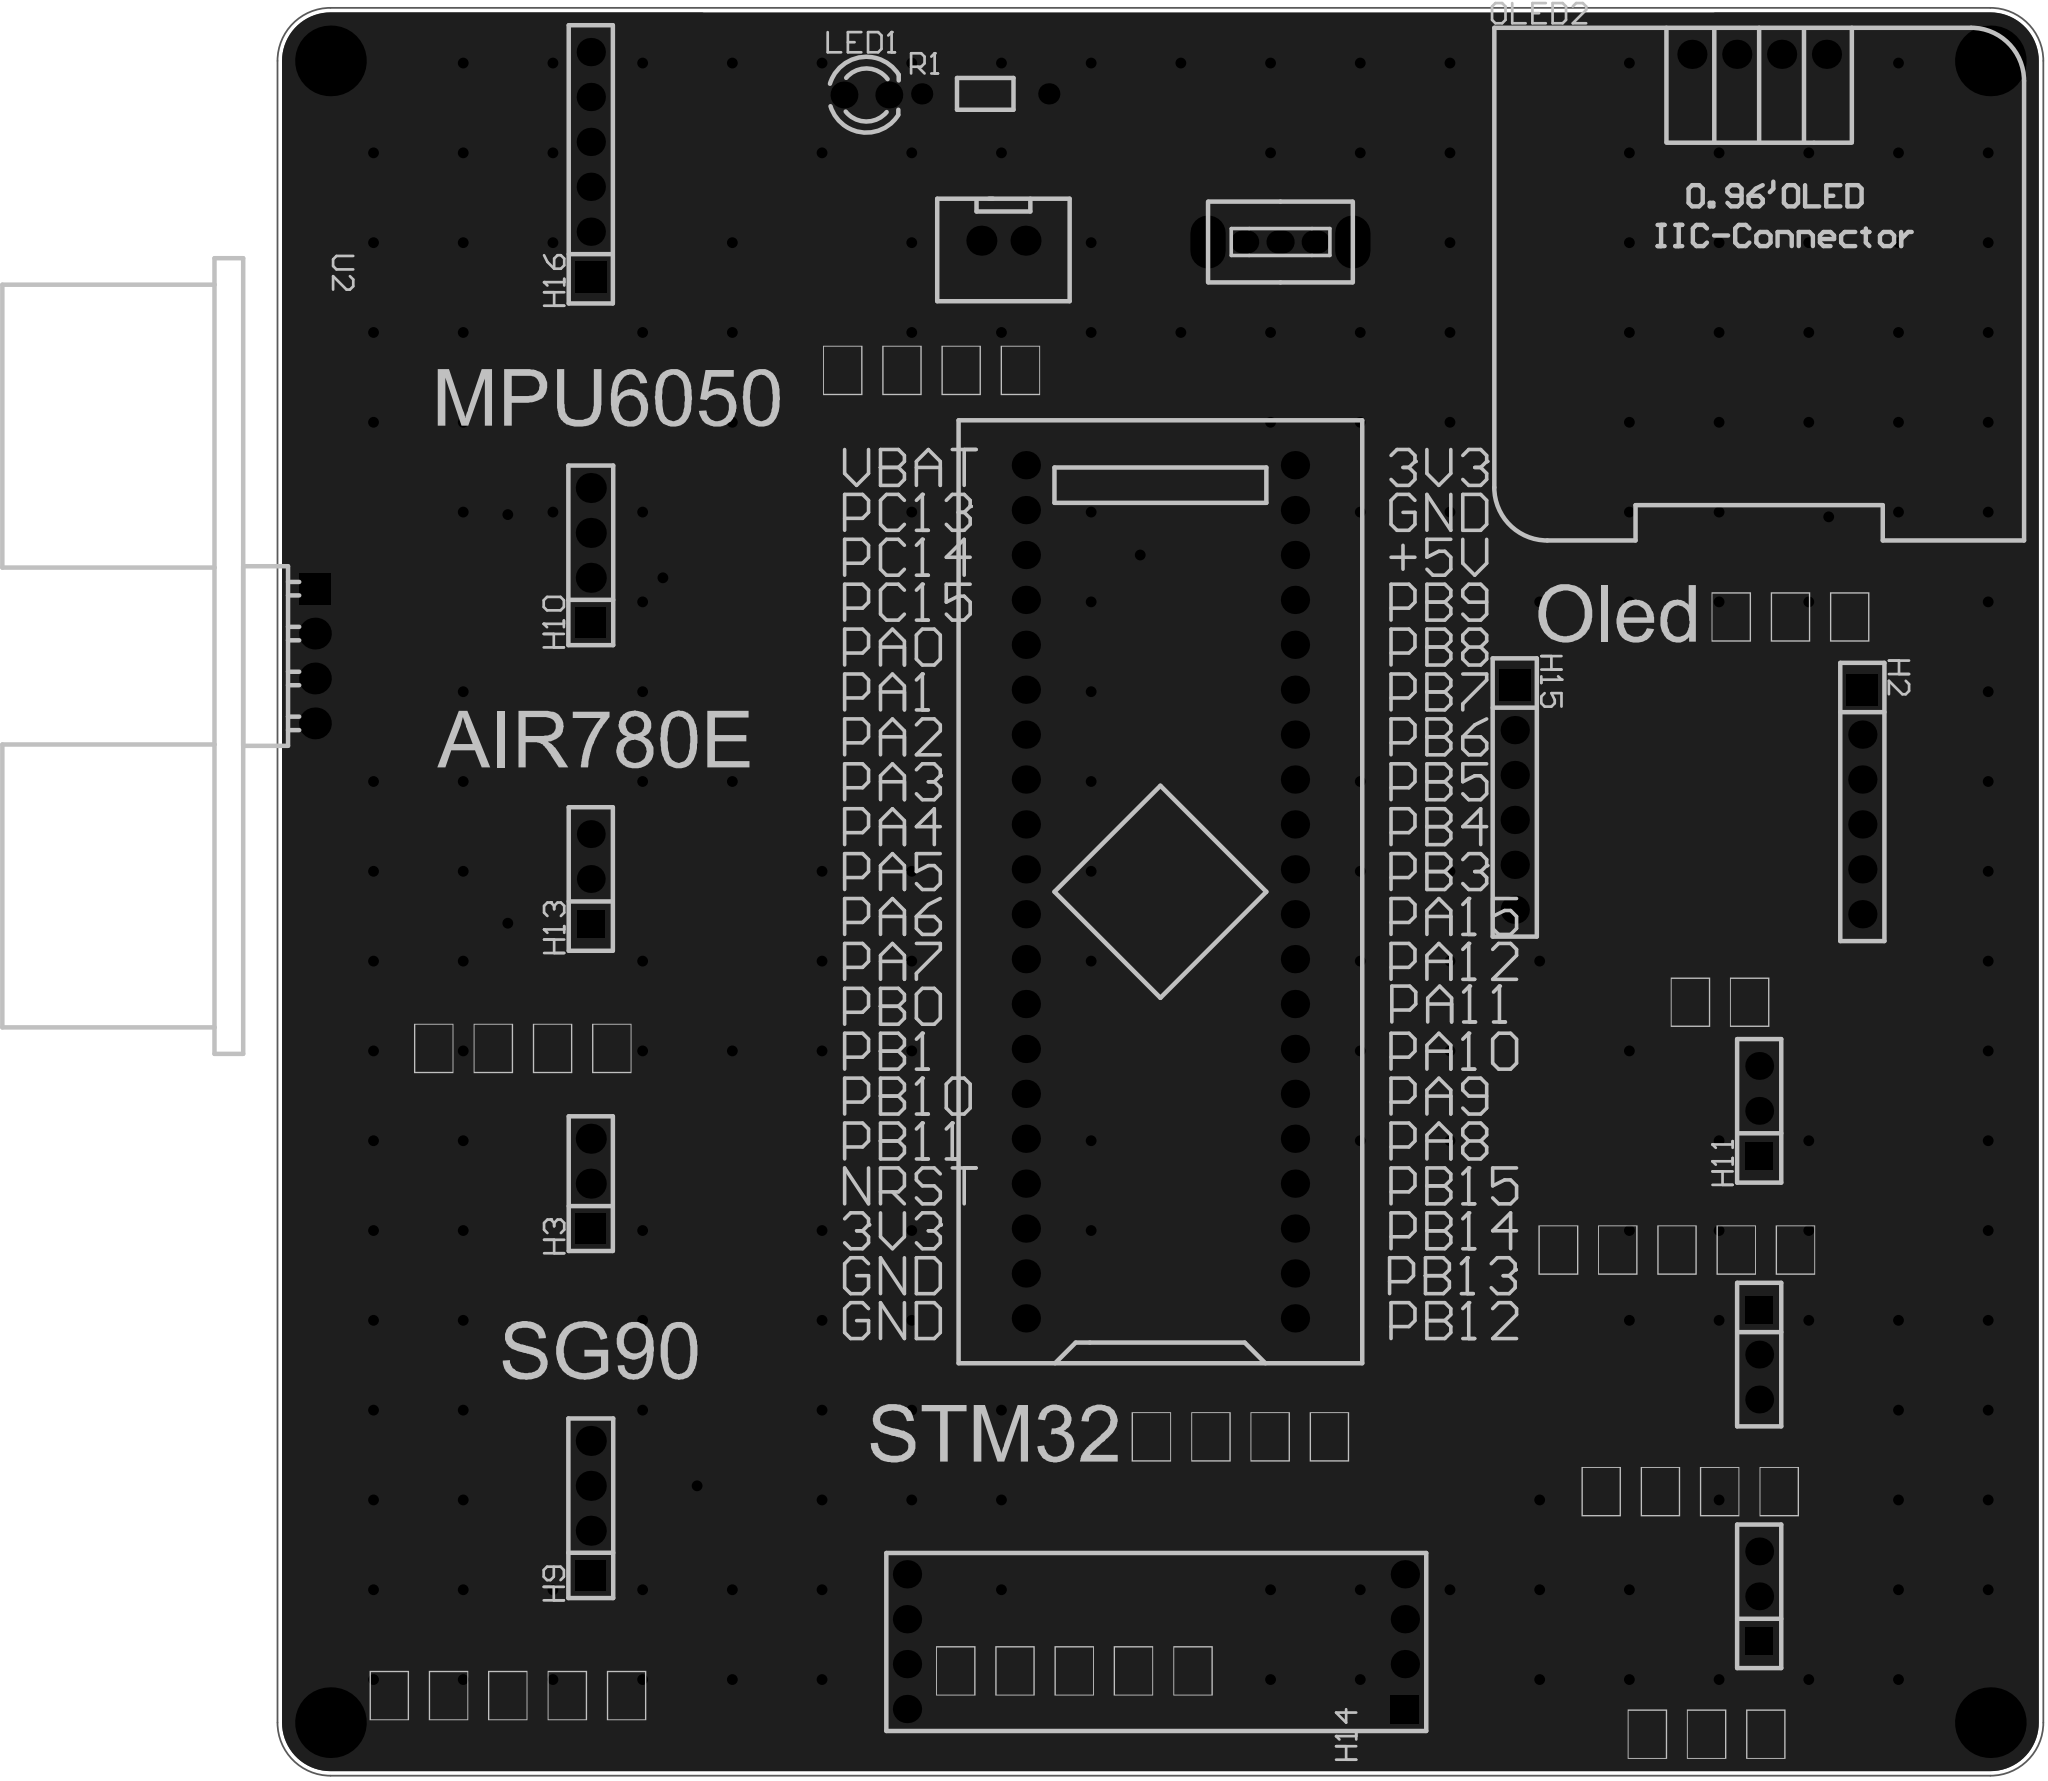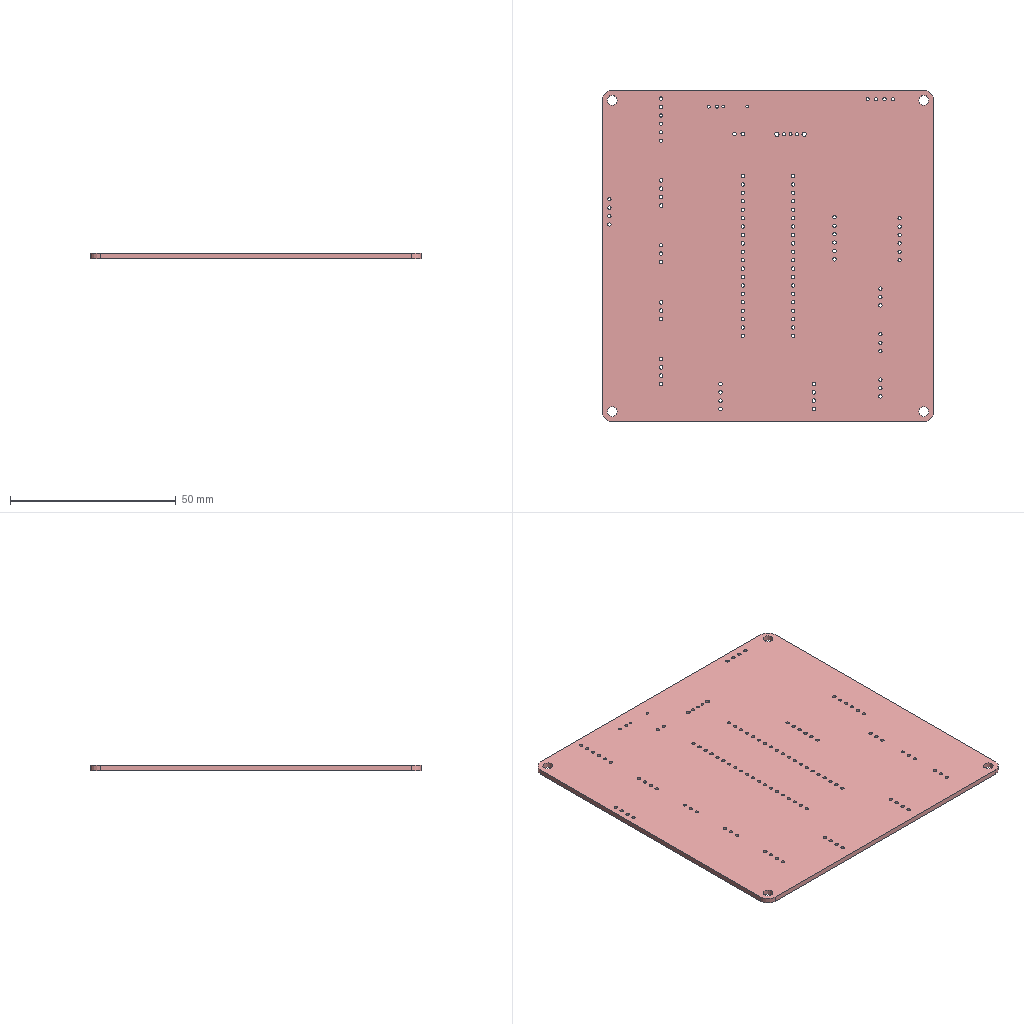Circuit board layout | Altium Designer | box 100 x 100 x 1.6 mm
Layer stack:
# Altium Designer layer stack of  (unit mm; dielectric type: 0 none, 1 core, 2 prepreg, 3 surface material)
index,name,kind,layer,copper_thickness_mm,dielectric_type,dielectric_thickness_mm,dielectric_material,dielectric_constant
0,Top Paste Mask Layer,other,,,,,,
1,Top Silkscreen Layer,other,,,,,,
2,Top Solder Mask Layer,dielectric,,,3,0.01,,3.3
3,Top Layer,copper,Top Layer,0.035,,,,
4,Dielectric1,dielectric,,,3,1.51,FR4,4.5
5,Bottom Layer,copper,Bottom Layer,0.035,,,,
6,Bottom Solder Mask Layer,dielectric,,,3,0.01,,3.3
7,Bottom Silkscreen Layer,other,,,,,,
8,Bottom Paste Mask Layer,other,,,,,,
# drill layer pairs: low layer,high layer
drill_pair,Top Layer,Bottom Layer
Part placement:
Designator,Comment,Layer,Footprint,Center-X(mm),Center-Y(mm),Rotation
U1,STM32F103C8T6-Card,TopLayer,CONN-TH_L53.3-W22.9_STM32F103C8T6-CARD,141.839,130.937,90
H12,,TopLayer,HDR-TH_3P-P2.54-V-F,175.748,104.757,270
CN4,XH2.54*2P_直插,TopLayer,CONN-TH_2P-P2.50-XH2.54-2P,132.949,167.767,0
SW5,,TopLayer,拨动开关,148.636,167.692,180
H1,,TopLayer,HDR-TH_3P-P2.54-V-F,175.748,91.083,90
OLED2,,TopLayer,0.96OLED_4P,175.748,178.308,0
H9,,TopLayer,HDR-TH_4P-P2.54-V-M,109.581,96.064,90
H10,,TopLayer,HDR-TH_4P-P2.54-V-M,109.581,149.967,90
H11,,TopLayer,HDR-TH_3P-P2.54-V-F,175.748,118.545,90
H13,,TopLayer,HDR-TH_3P-P2.54-V-F,109.581,131.659,90
H14,,TopLayer,HDR-TH_8P-P2.54-V-F-R2-C4-S2.54-1,141.585,88.519,90
H15,,TopLayer,HDR-TH_6P-P2.54-V-F,161.905,136.271,270
H16,,TopLayer,HDR-TH_6P-P2.54-V-F,109.581,172.085,90
LED1,,TopLayer,LED_TH-3mm,125.188,176.01,0
R1,100,TopLayer,Res_1/8W,131.919,176.072,0
U2,HC-SR04,TopLayer,TH_HC-SR04V,93.96,144.272,270
H2,,TopLayer,HDR-TH_6P-P2.54-V-F,181.59,136.017,270
H3,,TopLayer,HDR-TH_3P-P2.54-V-M,109.581,114.427,90
Pad and via stacks:
# Altium Designer via and pad stacks of  (unit mm). Each distinct definition once, with the count of objects using it.
# via: kind,start_layer,end_layer,hole_mm,diameter_mm,mode(0 simple;1 top-mid-bottom;2 full stack),diameter_per_layer,count,example_net
# pad: kind,layer,hole_mm,hole_type(0 round;1 square;2 slot),plating,top_size,top_shape(1 round;2 rect;3 octagon;9 rounded rect),mid_size,bottom_size,mode,footprint,size_per_layer,count,example
pad,Multi-Layer,3,0,plated,4x4,1,4x4,4x4,0,,,4,1
pad,Multi-Layer,1,0,plated,1.6x1.6,1,1.6x1.6,1.6x1.6,0,CONN-TH_L53.3-W22.9_STM32F103C8T6-CARD,,40,U1.1
pad,Multi-Layer,1.02,0,plated,1.575x1.575,1,1.575x1.575,1.575x1.575,0,HDR-TH_3P-P2.54-V-F,,8,H12.3
pad,Multi-Layer,1.02,0,plated,1.575x1.575,2,1.575x1.575,1.575x1.575,0,HDR-TH_3P-P2.54-V-F,,4,H12.1
pad,Multi-Layer,1.05,0,plated,1.7x1.7,1,1.7x1.7,1.7x1.7,0,CONN-TH_2P-P2.50-XH2.54-2P,,2,CN4.2
pad,Multi-Layer,0.8992,0,plated,1.6x1.3,1,1.6x1.3,1.6x1.3,0,\u00B2\u00A6\u00B6\u00AF\u00BF\u00AA\u00B9\u00D8,,3,SW5.1
pad,Multi-Layer,1.3,0,plated,3x1.999,1,3x1.999,3x1.999,0,\u00B2\u00A6\u00B6\u00AF\u00BF\u00AA\u00B9\u00D8,,2,SW5.4
pad,Multi-Layer,1,0,plated,1.65x1.65,1,1.65x1.65,1.65x1.65,0,0.96OLED_4P,,4,OLED2.4
pad,Multi-Layer,1.1,0,plated,1.7x1.7,2,1.7x1.7,1.7x1.7,0,HDR-TH_4P-P2.54-V-M,,2,H9.1
pad,Multi-Layer,1.1,0,plated,1.7x1.7,1,1.7x1.7,1.7x1.7,0,HDR-TH_4P-P2.54-V-M,,6,H9.2
pad,Multi-Layer,1.1,0,plated,1.6x1.6,2,1.6x1.6,1.6x1.6,0,HDR-TH_8P-P2.54-V-F-R2-C4-S2.54-1,,1,H14.1
pad,Multi-Layer,1.1,0,plated,1.6x1.6,1,1.6x1.6,1.6x1.6,0,HDR-TH_8P-P2.54-V-F-R2-C4-S2.54-1,,7,H14.2
pad,Multi-Layer,1.02,0,plated,1.6x1.6,1,1.6x1.6,1.6x1.6,0,HDR-TH_6P-P2.54-V-F,,15,H15.6
pad,Multi-Layer,1.02,0,plated,1.8x1.8,2,1.8x1.8,1.8x1.8,0,HDR-TH_6P-P2.54-V-F,,3,H15.1
pad,Multi-Layer,0.9144,0,plated,1.524x1.524,1,1.524x1.524,1.524x1.524,0,LED_TH-3mm,,2,LED1.1
pad,Multi-Layer,0.8001,0,plated,1.199x1.199,1,1.199x1.199,1.199x1.199,0,Res_1/8W,,2,R1.1
pad,Multi-Layer,1.001,0,plated,1.8x1.8,1,1.8x1.8,1.8x1.8,0,TH_HC-SR04V,,3,U2.4
pad,Multi-Layer,1.001,0,plated,1.8x1.8,2,1.8x1.8,1.8x1.8,0,TH_HC-SR04V,,1,U2.1
pad,Multi-Layer,1.1,0,plated,1.7x1.7,2,1.7x1.7,1.7x1.7,0,HDR-TH_3P-P2.54-V-M,,1,H3.1
pad,Multi-Layer,1.1,0,plated,1.7x1.7,1,1.7x1.7,1.7x1.7,0,HDR-TH_3P-P2.54-V-M,,2,H3.2
via,Top Layer,Bottom Layer,0.3048,0.61,0,,202,+5V
Copper pours:
name,layer,net,type(0 solid;1 hatched;2 none)
Bottom Layer-GND,Bottom Layer,GND,0
Top Layer-GND,Top Layer,GND,0
Design rules, without the lines most boards share:
# Altium Designer design rules of  (exported by Altium Designer, unit mm)
# columns: name | kind | enabled | priority | scope1 | scope2 | descriptor | typed fields (field=value)
Copper_copperRegion_copperThickness1oz | 0 | disabled | 4 | All | All | Clearance Constraint (Gap=5.984mil) (Disabled)(All),(All) | gap=0.152
Copper_copperRegion_copperThickness1oz_1 | 63 | disabled | 4 | All | All | Board Clearance Constraint (Gap=0mil) (Disabled)(All) |
Copper_copperRegion_Copper_copperRegion | 0 | disabled | 5 | All | All | Clearance Constraint (Gap=5.984mil) (Disabled)(All),(All) | gap=0.152
Copper_copperRegion_Copper_copperRegion_1 | 63 | disabled | 5 | All | All | Board Clearance Constraint (Gap=0mil) (Disabled)(All) |
copperThickness1oz | 0 | enabled | 6 | All | All | Clearance Constraint (Gap=5.984mil) (All),(All) | gap=0.152
copperThickness1oz_1 | 63 | enabled | 6 | All | All | Board Clearance Constraint (Gap=0mil) (All) |
copperRegion_copperThickness1oz | 20 | disabled | 1 | All | All | Polygon Connect Rule(Relief Connect )(Conductor Width=10mil) (Relief Angle=90 Angle) (Entries=4) (Air Gap Width=10mil) (Disabled)(All),(All) | connect_style(0=relief,1=direct,2=none)=0 relief_conductor_width=0.254 relief_entries=4
copperRegion_Copper_copperRegion | 20 | disabled | 2 | All | All | Polygon Connect Rule(Relief Connect )(Conductor Width=10mil) (Relief Angle=90 Angle) (Entries=4) (Air Gap Width=10mil) (Disabled)(All),(All) | connect_style(0=relief,1=direct,2=none)=0 relief_conductor_width=0.254 relief_entries=4
copperRegion | 20 | enabled | 3 | All | All | Polygon Connect Rule(Relief Connect )(Conductor Width=10mil) (Relief Angle=90 Angle) (Entries=4) (Air Gap Width=10mil) (All),(All) | connect_style(0=relief,1=direct,2=none)=0 relief_conductor_width=0.254 relief_entries=4